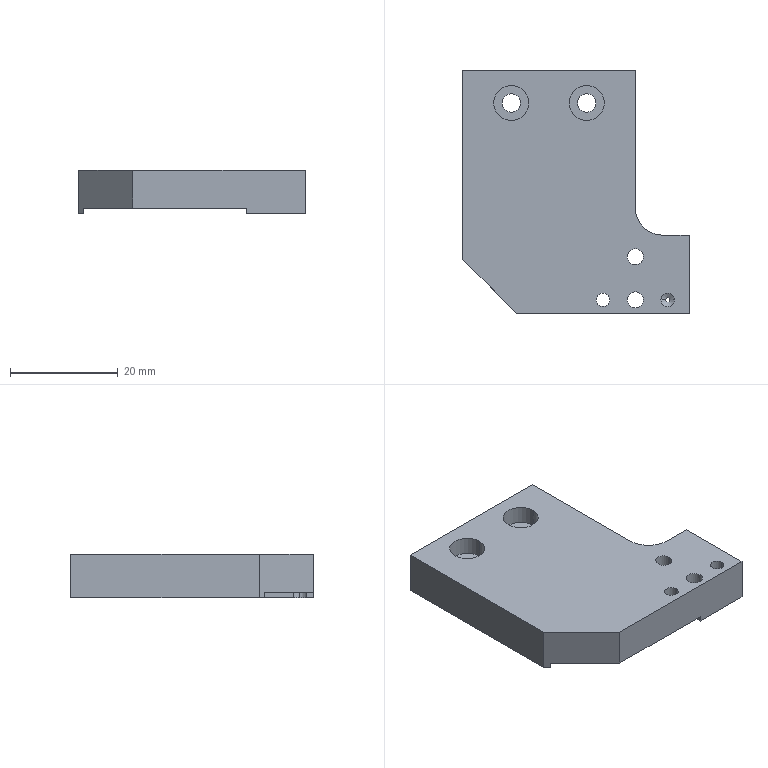Part | STEP file | 11-FG-E01811 | 1 solid | 36 faces | box 42 x 45 x 8 mm | volume 10535 mm3 | cylinder 17 | plane 17 | cone 2 | commonest cylinder face diameters 2.5 x4 3 x4 3.4 x4 6.5 x4 10 x1
STEP:
#1=CARTESIAN_POINT('',(8.75,-20.,1.));
#2=VERTEX_POINT('',#1);
#3=CARTESIAN_POINT('',(11.25,-20.,1.));
#4=VERTEX_POINT('',#3);
#5=CARTESIAN_POINT('',(10.,-20.,1.));
#6=DIRECTION('',(0.,0.,1.));
#7=DIRECTION('',(1.,0.,0.));
#8=AXIS2_PLACEMENT_3D('',#5,#6,#7);
#9=CIRCLE('',#8,1.25);
#10=EDGE_CURVE('',#2,#4,#9,.T.);
#11=ORIENTED_EDGE('',*,*,#10,.F.);
#12=CARTESIAN_POINT('',(8.75,-20.,8.));
#13=VERTEX_POINT('',#12);
#14=CARTESIAN_POINT('',(8.75,-20.,8.));
#15=DIRECTION('',(0.,0.,1.));
#16=VECTOR('',#15,1000.);
#17=LINE('',#14,#16);
#18=EDGE_CURVE('',#2,#13,#17,.T.);
#19=ORIENTED_EDGE('',*,*,#18,.T.);
#20=CARTESIAN_POINT('',(11.25,-20.,8.));
#21=VERTEX_POINT('',#20);
#22=CARTESIAN_POINT('',(10.,-20.,8.));
#23=DIRECTION('',(0.,0.,1.));
#24=DIRECTION('',(1.,0.,0.));
#25=AXIS2_PLACEMENT_3D('',#22,#23,#24);
#26=CIRCLE('',#25,1.25);
#27=EDGE_CURVE('',#13,#21,#26,.T.);
#28=ORIENTED_EDGE('',*,*,#27,.T.);
#29=CARTESIAN_POINT('',(11.25,-20.,8.));
#30=DIRECTION('',(0.,0.,1.));
#31=VECTOR('',#30,1000.);
#32=LINE('',#29,#31);
#33=EDGE_CURVE('',#4,#21,#32,.T.);
#34=ORIENTED_EDGE('',*,*,#33,.F.);
#35=EDGE_LOOP('',(#11,#19,#28,#34));
#36=FACE_OUTER_BOUND('',#35,.T.);
#37=CARTESIAN_POINT('',(10.,-20.,8.));
#38=DIRECTION('',(0.,0.,1.));
#39=DIRECTION('',(1.,0.,0.));
#40=AXIS2_PLACEMENT_3D('',#37,#38,#39);
#41=CYLINDRICAL_SURFACE('',#40,1.25);
#42=ADVANCED_FACE('',(#36),#41,.F.);
#43=CARTESIAN_POINT('',(20.75,-20.,0.5));
#44=VERTEX_POINT('',#43);
#45=CARTESIAN_POINT('',(23.25,-20.,0.5));
#46=VERTEX_POINT('',#45);
#47=CARTESIAN_POINT('',(22.,-20.,0.5));
#48=DIRECTION('',(0.,0.,1.));
#49=DIRECTION('',(1.,0.,0.));
#50=AXIS2_PLACEMENT_3D('',#47,#48,#49);
#51=CIRCLE('',#50,1.25);
#52=EDGE_CURVE('',#44,#46,#51,.T.);
#53=ORIENTED_EDGE('',*,*,#52,.F.);
#54=CARTESIAN_POINT('',(20.75,-20.,8.));
#55=VERTEX_POINT('',#54);
#56=CARTESIAN_POINT('',(20.75,-20.,8.));
#57=DIRECTION('',(0.,0.,1.));
#58=VECTOR('',#57,1000.);
#59=LINE('',#56,#58);
#60=EDGE_CURVE('',#44,#55,#59,.T.);
#61=ORIENTED_EDGE('',*,*,#60,.T.);
#62=CARTESIAN_POINT('',(23.25,-20.,8.));
#63=VERTEX_POINT('',#62);
#64=CARTESIAN_POINT('',(22.,-20.,8.));
#65=DIRECTION('',(0.,0.,1.));
#66=DIRECTION('',(1.,0.,0.));
#67=AXIS2_PLACEMENT_3D('',#64,#65,#66);
#68=CIRCLE('',#67,1.25);
#69=EDGE_CURVE('',#55,#63,#68,.T.);
#70=ORIENTED_EDGE('',*,*,#69,.T.);
#71=CARTESIAN_POINT('',(23.25,-20.,8.));
#72=DIRECTION('',(0.,0.,1.));
#73=VECTOR('',#72,1000.);
#74=LINE('',#71,#73);
#75=EDGE_CURVE('',#46,#63,#74,.T.);
#76=ORIENTED_EDGE('',*,*,#75,.F.);
#77=EDGE_LOOP('',(#53,#61,#70,#76));
#78=FACE_OUTER_BOUND('',#77,.T.);
#79=CARTESIAN_POINT('',(22.,-20.,8.));
#80=DIRECTION('',(0.,0.,1.));
#81=DIRECTION('',(1.,0.,0.));
#82=AXIS2_PLACEMENT_3D('',#79,#80,#81);
#83=CYLINDRICAL_SURFACE('',#82,1.25);
#84=ADVANCED_FACE('',(#78),#83,.F.);
#85=CARTESIAN_POINT('',(22.418,-20.,0.));
#86=VERTEX_POINT('',#85);
#87=CARTESIAN_POINT('',(21.582,-20.,0.));
#88=VERTEX_POINT('',#87);
#89=CARTESIAN_POINT('',(22.,-20.,0.));
#90=DIRECTION('',(0.,0.,-1.));
#91=DIRECTION('',(-1.,0.,0.));
#92=AXIS2_PLACEMENT_3D('',#89,#90,#91);
#93=CIRCLE('',#92,0.4179);
#94=EDGE_CURVE('',#86,#88,#93,.T.);
#95=ORIENTED_EDGE('',*,*,#94,.T.);
#96=CARTESIAN_POINT('',(20.75,-20.,0.5));
#97=DIRECTION('',(-0.8572,0.,0.515));
#98=VECTOR('',#97,1000.);
#99=LINE('',#96,#98);
#100=EDGE_CURVE('',#88,#44,#99,.T.);
#101=ORIENTED_EDGE('',*,*,#100,.T.);
#102=ORIENTED_EDGE('',*,*,#52,.T.);
#103=CARTESIAN_POINT('',(23.25,-20.,0.5));
#104=DIRECTION('',(0.8572,0.,0.515));
#105=VECTOR('',#104,1000.);
#106=LINE('',#103,#105);
#107=EDGE_CURVE('',#86,#46,#106,.T.);
#108=ORIENTED_EDGE('',*,*,#107,.F.);
#109=EDGE_LOOP('',(#95,#101,#102,#108));
#110=FACE_OUTER_BOUND('',#109,.T.);
#111=CARTESIAN_POINT('',(22.,-20.,0.5));
#112=DIRECTION('',(0.,0.,1.));
#113=DIRECTION('',(1.,0.,0.));
#114=AXIS2_PLACEMENT_3D('',#111,#112,#113);
#115=CONICAL_SURFACE('',#114,1.25,1.03);
#116=ADVANCED_FACE('',(#110),#115,.F.);
#117=CARTESIAN_POINT('',(14.5,-12.,1.));
#118=VERTEX_POINT('',#117);
#119=CARTESIAN_POINT('',(15.05,-13.161,1.));
#120=VERTEX_POINT('',#119);
#121=CARTESIAN_POINT('',(16.,-12.,1.));
#122=DIRECTION('',(0.,0.,1.));
#123=DIRECTION('',(1.,0.,0.));
#124=AXIS2_PLACEMENT_3D('',#121,#122,#123);
#125=CIRCLE('',#124,1.5);
#126=EDGE_CURVE('',#118,#120,#125,.T.);
#127=ORIENTED_EDGE('',*,*,#126,.F.);
#128=CARTESIAN_POINT('',(14.5,-12.,8.));
#129=VERTEX_POINT('',#128);
#130=CARTESIAN_POINT('',(14.5,-12.,8.));
#131=DIRECTION('',(0.,0.,1.));
#132=VECTOR('',#131,1000.);
#133=LINE('',#130,#132);
#134=EDGE_CURVE('',#118,#129,#133,.T.);
#135=ORIENTED_EDGE('',*,*,#134,.T.);
#136=CARTESIAN_POINT('',(17.5,-12.,8.));
#137=VERTEX_POINT('',#136);
#138=CARTESIAN_POINT('',(16.,-12.,8.));
#139=DIRECTION('',(0.,0.,1.));
#140=DIRECTION('',(1.,0.,0.));
#141=AXIS2_PLACEMENT_3D('',#138,#139,#140);
#142=CIRCLE('',#141,1.5);
#143=EDGE_CURVE('',#129,#137,#142,.T.);
#144=ORIENTED_EDGE('',*,*,#143,.T.);
#145=CARTESIAN_POINT('',(17.5,-12.,0.));
#146=VERTEX_POINT('',#145);
#147=CARTESIAN_POINT('',(17.5,-12.,8.));
#148=DIRECTION('',(0.,0.,1.));
#149=VECTOR('',#148,1000.);
#150=LINE('',#147,#149);
#151=EDGE_CURVE('',#146,#137,#150,.T.);
#152=ORIENTED_EDGE('',*,*,#151,.F.);
#153=CARTESIAN_POINT('',(15.05,-13.161,0.));
#154=VERTEX_POINT('',#153);
#155=CARTESIAN_POINT('',(16.,-12.,0.));
#156=DIRECTION('',(0.,0.,-1.));
#157=DIRECTION('',(-1.,0.,0.));
#158=AXIS2_PLACEMENT_3D('',#155,#156,#157);
#159=CIRCLE('',#158,1.5);
#160=EDGE_CURVE('',#146,#154,#159,.T.);
#161=ORIENTED_EDGE('',*,*,#160,.T.);
#162=CARTESIAN_POINT('',(15.05,-13.161,8.));
#163=DIRECTION('',(0.,0.,-1.));
#164=VECTOR('',#163,1000.);
#165=LINE('',#162,#164);
#166=EDGE_CURVE('',#120,#154,#165,.T.);
#167=ORIENTED_EDGE('',*,*,#166,.F.);
#168=EDGE_LOOP('',(#127,#135,#144,#152,#161,#167));
#169=FACE_OUTER_BOUND('',#168,.T.);
#170=CARTESIAN_POINT('',(16.,-12.,8.));
#171=DIRECTION('',(0.,0.,1.));
#172=DIRECTION('',(1.,0.,0.));
#173=AXIS2_PLACEMENT_3D('',#170,#171,#172);
#174=CYLINDRICAL_SURFACE('',#173,1.5);
#175=ADVANCED_FACE('',(#169),#174,.F.);
#176=CARTESIAN_POINT('',(14.5,-20.,1.));
#177=VERTEX_POINT('',#176);
#178=CARTESIAN_POINT('',(15.05,-21.161,1.));
#179=VERTEX_POINT('',#178);
#180=CARTESIAN_POINT('',(16.,-20.,1.));
#181=DIRECTION('',(0.,0.,1.));
#182=DIRECTION('',(1.,0.,0.));
#183=AXIS2_PLACEMENT_3D('',#180,#181,#182);
#184=CIRCLE('',#183,1.5);
#185=EDGE_CURVE('',#177,#179,#184,.T.);
#186=ORIENTED_EDGE('',*,*,#185,.F.);
#187=CARTESIAN_POINT('',(14.5,-20.,8.));
#188=VERTEX_POINT('',#187);
#189=CARTESIAN_POINT('',(14.5,-20.,8.));
#190=DIRECTION('',(0.,0.,1.));
#191=VECTOR('',#190,1000.);
#192=LINE('',#189,#191);
#193=EDGE_CURVE('',#177,#188,#192,.T.);
#194=ORIENTED_EDGE('',*,*,#193,.T.);
#195=CARTESIAN_POINT('',(17.5,-20.,8.));
#196=VERTEX_POINT('',#195);
#197=CARTESIAN_POINT('',(16.,-20.,8.));
#198=DIRECTION('',(0.,0.,1.));
#199=DIRECTION('',(1.,0.,0.));
#200=AXIS2_PLACEMENT_3D('',#197,#198,#199);
#201=CIRCLE('',#200,1.5);
#202=EDGE_CURVE('',#188,#196,#201,.T.);
#203=ORIENTED_EDGE('',*,*,#202,.T.);
#204=CARTESIAN_POINT('',(17.5,-20.,0.));
#205=VERTEX_POINT('',#204);
#206=CARTESIAN_POINT('',(17.5,-20.,8.));
#207=DIRECTION('',(0.,0.,1.));
#208=VECTOR('',#207,1000.);
#209=LINE('',#206,#208);
#210=EDGE_CURVE('',#205,#196,#209,.T.);
#211=ORIENTED_EDGE('',*,*,#210,.F.);
#212=CARTESIAN_POINT('',(15.05,-21.161,0.));
#213=VERTEX_POINT('',#212);
#214=CARTESIAN_POINT('',(16.,-20.,0.));
#215=DIRECTION('',(0.,0.,-1.));
#216=DIRECTION('',(-1.,0.,0.));
#217=AXIS2_PLACEMENT_3D('',#214,#215,#216);
#218=CIRCLE('',#217,1.5);
#219=EDGE_CURVE('',#205,#213,#218,.T.);
#220=ORIENTED_EDGE('',*,*,#219,.T.);
#221=CARTESIAN_POINT('',(15.05,-21.161,8.));
#222=DIRECTION('',(0.,0.,-1.));
#223=VECTOR('',#222,1000.);
#224=LINE('',#221,#223);
#225=EDGE_CURVE('',#179,#213,#224,.T.);
#226=ORIENTED_EDGE('',*,*,#225,.F.);
#227=EDGE_LOOP('',(#186,#194,#203,#211,#220,#226));
#228=FACE_OUTER_BOUND('',#227,.T.);
#229=CARTESIAN_POINT('',(16.,-20.,8.));
#230=DIRECTION('',(0.,0.,1.));
#231=DIRECTION('',(1.,0.,0.));
#232=AXIS2_PLACEMENT_3D('',#229,#230,#231);
#233=CYLINDRICAL_SURFACE('',#232,1.5);
#234=ADVANCED_FACE('',(#228),#233,.F.);
#235=CARTESIAN_POINT('',(3.75,16.5,4.6));
#236=VERTEX_POINT('',#235);
#237=CARTESIAN_POINT('',(10.25,16.5,4.6));
#238=VERTEX_POINT('',#237);
#239=CARTESIAN_POINT('',(7.,16.5,4.6));
#240=DIRECTION('',(0.,0.,1.));
#241=DIRECTION('',(1.,0.,0.));
#242=AXIS2_PLACEMENT_3D('',#239,#240,#241);
#243=CIRCLE('',#242,3.25);
#244=EDGE_CURVE('',#236,#238,#243,.T.);
#245=ORIENTED_EDGE('',*,*,#244,.F.);
#246=CARTESIAN_POINT('',(3.75,16.5,8.));
#247=VERTEX_POINT('',#246);
#248=CARTESIAN_POINT('',(3.75,16.5,8.));
#249=DIRECTION('',(0.,0.,1.));
#250=VECTOR('',#249,1000.);
#251=LINE('',#248,#250);
#252=EDGE_CURVE('',#236,#247,#251,.T.);
#253=ORIENTED_EDGE('',*,*,#252,.T.);
#254=CARTESIAN_POINT('',(10.25,16.5,8.));
#255=VERTEX_POINT('',#254);
#256=CARTESIAN_POINT('',(7.,16.5,8.));
#257=DIRECTION('',(0.,0.,1.));
#258=DIRECTION('',(1.,0.,0.));
#259=AXIS2_PLACEMENT_3D('',#256,#257,#258);
#260=CIRCLE('',#259,3.25);
#261=EDGE_CURVE('',#247,#255,#260,.T.);
#262=ORIENTED_EDGE('',*,*,#261,.T.);
#263=CARTESIAN_POINT('',(10.25,16.5,8.));
#264=DIRECTION('',(0.,0.,1.));
#265=VECTOR('',#264,1000.);
#266=LINE('',#263,#265);
#267=EDGE_CURVE('',#238,#255,#266,.T.);
#268=ORIENTED_EDGE('',*,*,#267,.F.);
#269=EDGE_LOOP('',(#245,#253,#262,#268));
#270=FACE_OUTER_BOUND('',#269,.T.);
#271=CARTESIAN_POINT('',(7.,16.5,8.));
#272=DIRECTION('',(0.,0.,1.));
#273=DIRECTION('',(1.,0.,0.));
#274=AXIS2_PLACEMENT_3D('',#271,#272,#273);
#275=CYLINDRICAL_SURFACE('',#274,3.25);
#276=ADVANCED_FACE('',(#270),#275,.F.);
#277=CARTESIAN_POINT('',(5.3,16.5,1.));
#278=VERTEX_POINT('',#277);
#279=CARTESIAN_POINT('',(8.7,16.5,1.));
#280=VERTEX_POINT('',#279);
#281=CARTESIAN_POINT('',(7.,16.5,1.));
#282=DIRECTION('',(0.,0.,1.));
#283=DIRECTION('',(1.,0.,0.));
#284=AXIS2_PLACEMENT_3D('',#281,#282,#283);
#285=CIRCLE('',#284,1.7);
#286=EDGE_CURVE('',#278,#280,#285,.T.);
#287=ORIENTED_EDGE('',*,*,#286,.F.);
#288=CARTESIAN_POINT('',(5.3,16.5,4.6));
#289=VERTEX_POINT('',#288);
#290=CARTESIAN_POINT('',(5.3,16.5,8.));
#291=DIRECTION('',(0.,0.,1.));
#292=VECTOR('',#291,1000.);
#293=LINE('',#290,#292);
#294=EDGE_CURVE('',#278,#289,#293,.T.);
#295=ORIENTED_EDGE('',*,*,#294,.T.);
#296=CARTESIAN_POINT('',(8.7,16.5,4.6));
#297=VERTEX_POINT('',#296);
#298=CARTESIAN_POINT('',(7.,16.5,4.6));
#299=DIRECTION('',(0.,0.,1.));
#300=DIRECTION('',(1.,0.,0.));
#301=AXIS2_PLACEMENT_3D('',#298,#299,#300);
#302=CIRCLE('',#301,1.7);
#303=EDGE_CURVE('',#289,#297,#302,.T.);
#304=ORIENTED_EDGE('',*,*,#303,.T.);
#305=CARTESIAN_POINT('',(8.7,16.5,8.));
#306=DIRECTION('',(0.,0.,1.));
#307=VECTOR('',#306,1000.);
#308=LINE('',#305,#307);
#309=EDGE_CURVE('',#280,#297,#308,.T.);
#310=ORIENTED_EDGE('',*,*,#309,.F.);
#311=EDGE_LOOP('',(#287,#295,#304,#310));
#312=FACE_OUTER_BOUND('',#311,.T.);
#313=CARTESIAN_POINT('',(7.,16.5,8.));
#314=DIRECTION('',(0.,0.,1.));
#315=DIRECTION('',(1.,0.,0.));
#316=AXIS2_PLACEMENT_3D('',#313,#314,#315);
#317=CYLINDRICAL_SURFACE('',#316,1.7);
#318=ADVANCED_FACE('',(#312),#317,.F.);
#319=CARTESIAN_POINT('',(-10.25,16.5,4.6));
#320=VERTEX_POINT('',#319);
#321=CARTESIAN_POINT('',(-3.75,16.5,4.6));
#322=VERTEX_POINT('',#321);
#323=CARTESIAN_POINT('',(-7.,16.5,4.6));
#324=DIRECTION('',(0.,0.,1.));
#325=DIRECTION('',(1.,0.,0.));
#326=AXIS2_PLACEMENT_3D('',#323,#324,#325);
#327=CIRCLE('',#326,3.25);
#328=EDGE_CURVE('',#320,#322,#327,.T.);
#329=ORIENTED_EDGE('',*,*,#328,.F.);
#330=CARTESIAN_POINT('',(-10.25,16.5,8.));
#331=VERTEX_POINT('',#330);
#332=CARTESIAN_POINT('',(-10.25,16.5,8.));
#333=DIRECTION('',(0.,0.,1.));
#334=VECTOR('',#333,1000.);
#335=LINE('',#332,#334);
#336=EDGE_CURVE('',#320,#331,#335,.T.);
#337=ORIENTED_EDGE('',*,*,#336,.T.);
#338=CARTESIAN_POINT('',(-3.75,16.5,8.));
#339=VERTEX_POINT('',#338);
#340=CARTESIAN_POINT('',(-7.,16.5,8.));
#341=DIRECTION('',(0.,0.,1.));
#342=DIRECTION('',(1.,0.,0.));
#343=AXIS2_PLACEMENT_3D('',#340,#341,#342);
#344=CIRCLE('',#343,3.25);
#345=EDGE_CURVE('',#331,#339,#344,.T.);
#346=ORIENTED_EDGE('',*,*,#345,.T.);
#347=CARTESIAN_POINT('',(-3.75,16.5,8.));
#348=DIRECTION('',(0.,0.,1.));
#349=VECTOR('',#348,1000.);
#350=LINE('',#347,#349);
#351=EDGE_CURVE('',#322,#339,#350,.T.);
#352=ORIENTED_EDGE('',*,*,#351,.F.);
#353=EDGE_LOOP('',(#329,#337,#346,#352));
#354=FACE_OUTER_BOUND('',#353,.T.);
#355=CARTESIAN_POINT('',(-7.,16.5,8.));
#356=DIRECTION('',(0.,0.,1.));
#357=DIRECTION('',(1.,0.,0.));
#358=AXIS2_PLACEMENT_3D('',#355,#356,#357);
#359=CYLINDRICAL_SURFACE('',#358,3.25);
#360=ADVANCED_FACE('',(#354),#359,.F.);
#361=CARTESIAN_POINT('',(-8.7,16.5,1.));
#362=VERTEX_POINT('',#361);
#363=CARTESIAN_POINT('',(-5.3,16.5,1.));
#364=VERTEX_POINT('',#363);
#365=CARTESIAN_POINT('',(-7.,16.5,1.));
#366=DIRECTION('',(0.,0.,1.));
#367=DIRECTION('',(1.,0.,0.));
#368=AXIS2_PLACEMENT_3D('',#365,#366,#367);
#369=CIRCLE('',#368,1.7);
#370=EDGE_CURVE('',#362,#364,#369,.T.);
#371=ORIENTED_EDGE('',*,*,#370,.F.);
#372=CARTESIAN_POINT('',(-8.7,16.5,4.6));
#373=VERTEX_POINT('',#372);
#374=CARTESIAN_POINT('',(-8.7,16.5,8.));
#375=DIRECTION('',(0.,0.,1.));
#376=VECTOR('',#375,1000.);
#377=LINE('',#374,#376);
#378=EDGE_CURVE('',#362,#373,#377,.T.);
#379=ORIENTED_EDGE('',*,*,#378,.T.);
#380=CARTESIAN_POINT('',(-5.3,16.5,4.6));
#381=VERTEX_POINT('',#380);
#382=CARTESIAN_POINT('',(-7.,16.5,4.6));
#383=DIRECTION('',(0.,0.,1.));
#384=DIRECTION('',(1.,0.,0.));
#385=AXIS2_PLACEMENT_3D('',#382,#383,#384);
#386=CIRCLE('',#385,1.7);
#387=EDGE_CURVE('',#373,#381,#386,.T.);
#388=ORIENTED_EDGE('',*,*,#387,.T.);
#389=CARTESIAN_POINT('',(-5.3,16.5,8.));
#390=DIRECTION('',(0.,0.,1.));
#391=VECTOR('',#390,1000.);
#392=LINE('',#389,#391);
#393=EDGE_CURVE('',#364,#381,#392,.T.);
#394=ORIENTED_EDGE('',*,*,#393,.F.);
#395=EDGE_LOOP('',(#371,#379,#388,#394));
#396=FACE_OUTER_BOUND('',#395,.T.);
#397=CARTESIAN_POINT('',(-7.,16.5,8.));
#398=DIRECTION('',(0.,0.,1.));
#399=DIRECTION('',(1.,0.,0.));
#400=AXIS2_PLACEMENT_3D('',#397,#398,#399);
#401=CYLINDRICAL_SURFACE('',#400,1.7);
#402=ADVANCED_FACE('',(#396),#401,.F.);
#403=CARTESIAN_POINT('',(15.05,22.5,0.));
#404=VERTEX_POINT('',#403);
#405=CARTESIAN_POINT('',(15.05,-10.839,0.));
#406=VERTEX_POINT('',#405);
#407=CARTESIAN_POINT('',(15.05,0.,0.));
#408=DIRECTION('',(0.,-1.,0.));
#409=VECTOR('',#408,1000.);
#410=LINE('',#407,#409);
#411=EDGE_CURVE('',#404,#406,#410,.T.);
#412=ORIENTED_EDGE('',*,*,#411,.T.);
#413=CARTESIAN_POINT('',(15.05,-10.839,1.));
#414=VERTEX_POINT('',#413);
#415=CARTESIAN_POINT('',(15.05,-10.839,8.));
#416=DIRECTION('',(0.,0.,1.));
#417=VECTOR('',#416,1000.);
#418=LINE('',#415,#417);
#419=EDGE_CURVE('',#406,#414,#418,.T.);
#420=ORIENTED_EDGE('',*,*,#419,.T.);
#421=CARTESIAN_POINT('',(15.05,22.5,1.));
#422=VERTEX_POINT('',#421);
#423=CARTESIAN_POINT('',(15.05,-33.5,1.));
#424=DIRECTION('',(0.,1.,0.));
#425=VECTOR('',#424,1000.);
#426=LINE('',#423,#425);
#427=EDGE_CURVE('',#414,#422,#426,.T.);
#428=ORIENTED_EDGE('',*,*,#427,.T.);
#429=CARTESIAN_POINT('',(15.05,22.5,1.));
#430=DIRECTION('',(0.,0.,-1.));
#431=VECTOR('',#430,1000.);
#432=LINE('',#429,#431);
#433=EDGE_CURVE('',#422,#404,#432,.T.);
#434=ORIENTED_EDGE('',*,*,#433,.T.);
#435=EDGE_LOOP('',(#412,#420,#428,#434));
#436=FACE_OUTER_BOUND('',#435,.T.);
#437=CARTESIAN_POINT('',(15.05,-33.5,1.));
#438=DIRECTION('',(1.,0.,0.));
#439=DIRECTION('',(0.,0.,-1.));
#440=AXIS2_PLACEMENT_3D('',#437,#438,#439);
#441=PLANE('',#440);
#442=ADVANCED_FACE('',(#436),#441,.F.);
#443=CARTESIAN_POINT('',(15.05,-18.839,1.));
#444=VERTEX_POINT('',#443);
#445=CARTESIAN_POINT('',(15.05,-33.5,1.));
#446=DIRECTION('',(0.,1.,0.));
#447=VECTOR('',#446,1000.);
#448=LINE('',#445,#447);
#449=EDGE_CURVE('',#444,#120,#448,.T.);
#450=ORIENTED_EDGE('',*,*,#449,.T.);
#451=ORIENTED_EDGE('',*,*,#166,.T.);
#452=CARTESIAN_POINT('',(15.05,-18.839,0.));
#453=VERTEX_POINT('',#452);
#454=CARTESIAN_POINT('',(15.05,0.,0.));
#455=DIRECTION('',(0.,-1.,0.));
#456=VECTOR('',#455,1000.);
#457=LINE('',#454,#456);
#458=EDGE_CURVE('',#154,#453,#457,.T.);
#459=ORIENTED_EDGE('',*,*,#458,.T.);
#460=CARTESIAN_POINT('',(15.05,-18.839,8.));
#461=DIRECTION('',(0.,0.,1.));
#462=VECTOR('',#461,1000.);
#463=LINE('',#460,#462);
#464=EDGE_CURVE('',#453,#444,#463,.T.);
#465=ORIENTED_EDGE('',*,*,#464,.T.);
#466=EDGE_LOOP('',(#450,#451,#459,#465));
#467=FACE_OUTER_BOUND('',#466,.T.);
#468=CARTESIAN_POINT('',(15.05,-33.5,1.));
#469=DIRECTION('',(1.,0.,0.));
#470=DIRECTION('',(0.,0.,-1.));
#471=AXIS2_PLACEMENT_3D('',#468,#469,#470);
#472=PLANE('',#471);
#473=ADVANCED_FACE('',(#467),#472,.F.);
#474=CARTESIAN_POINT('',(16.,-3.,8.));
#475=VERTEX_POINT('',#474);
#476=CARTESIAN_POINT('',(16.,22.5,8.));
#477=VERTEX_POINT('',#476);
#478=CARTESIAN_POINT('',(16.,-22.5,8.));
#479=DIRECTION('',(0.,1.,0.));
#480=VECTOR('',#479,1000.);
#481=LINE('',#478,#480);
#482=EDGE_CURVE('',#475,#477,#481,.T.);
#483=ORIENTED_EDGE('',*,*,#482,.F.);
#484=CARTESIAN_POINT('',(16.,-3.,0.));
#485=VERTEX_POINT('',#484);
#486=CARTESIAN_POINT('',(16.,-3.,8.));
#487=DIRECTION('',(0.,0.,-1.));
#488=VECTOR('',#487,1000.);
#489=LINE('',#486,#488);
#490=EDGE_CURVE('',#475,#485,#489,.T.);
#491=ORIENTED_EDGE('',*,*,#490,.T.);
#492=CARTESIAN_POINT('',(16.,22.5,0.));
#493=VERTEX_POINT('',#492);
#494=CARTESIAN_POINT('',(16.,-22.5,0.));
#495=DIRECTION('',(0.,1.,0.));
#496=VECTOR('',#495,1000.);
#497=LINE('',#494,#496);
#498=EDGE_CURVE('',#485,#493,#497,.T.);
#499=ORIENTED_EDGE('',*,*,#498,.T.);
#500=CARTESIAN_POINT('',(16.,22.5,8.));
#501=DIRECTION('',(0.,0.,-1.));
#502=VECTOR('',#501,1000.);
#503=LINE('',#500,#502);
#504=EDGE_CURVE('',#477,#493,#503,.T.);
#505=ORIENTED_EDGE('',*,*,#504,.F.);
#506=EDGE_LOOP('',(#483,#491,#499,#505));
#507=FACE_OUTER_BOUND('',#506,.T.);
#508=CARTESIAN_POINT('',(16.,-22.5,8.));
#509=DIRECTION('',(-1.,0.,0.));
#510=DIRECTION('',(0.,0.,1.));
#511=AXIS2_PLACEMENT_3D('',#508,#509,#510);
#512=PLANE('',#511);
#513=ADVANCED_FACE('',(#507),#512,.F.);
#514=ORIENTED_EDGE('',*,*,#94,.F.);
#515=CARTESIAN_POINT('',(22.,-20.,0.));
#516=DIRECTION('',(0.,0.,-1.));
#517=DIRECTION('',(-1.,0.,0.));
#518=AXIS2_PLACEMENT_3D('',#515,#516,#517);
#519=CIRCLE('',#518,0.4179);
#520=EDGE_CURVE('',#88,#86,#519,.T.);
#521=ORIENTED_EDGE('',*,*,#520,.F.);
#522=EDGE_LOOP('',(#514,#521));
#523=FACE_BOUND('',#522,.T.);
#524=CARTESIAN_POINT('',(16.,-12.,0.));
#525=DIRECTION('',(0.,0.,-1.));
#526=DIRECTION('',(-1.,0.,0.));
#527=AXIS2_PLACEMENT_3D('',#524,#525,#526);
#528=CIRCLE('',#527,1.5);
#529=EDGE_CURVE('',#406,#146,#528,.T.);
#530=ORIENTED_EDGE('',*,*,#529,.F.);
#531=ORIENTED_EDGE('',*,*,#411,.F.);
#532=CARTESIAN_POINT('',(-16.,22.5,0.));
#533=DIRECTION('',(-1.,0.,0.));
#534=VECTOR('',#533,1000.);
#535=LINE('',#532,#534);
#536=EDGE_CURVE('',#493,#404,#535,.T.);
#537=ORIENTED_EDGE('',*,*,#536,.F.);
#538=ORIENTED_EDGE('',*,*,#498,.F.);
#539=CARTESIAN_POINT('',(21.,-8.,0.));
#540=VERTEX_POINT('',#539);
#541=CARTESIAN_POINT('',(21.,-3.,0.));
#542=DIRECTION('',(0.,0.,1.));
#543=DIRECTION('',(-1.,0.,0.));
#544=AXIS2_PLACEMENT_3D('',#541,#542,#543);
#545=CIRCLE('',#544,5.);
#546=EDGE_CURVE('',#485,#540,#545,.T.);
#547=ORIENTED_EDGE('',*,*,#546,.T.);
#548=CARTESIAN_POINT('',(26.,-8.,0.));
#549=VERTEX_POINT('',#548);
#550=CARTESIAN_POINT('',(16.,-8.,0.));
#551=DIRECTION('',(-1.,0.,0.));
#552=VECTOR('',#551,1000.);
#553=LINE('',#550,#552);
#554=EDGE_CURVE('',#549,#540,#553,.T.);
#555=ORIENTED_EDGE('',*,*,#554,.F.);
#556=CARTESIAN_POINT('',(26.,-22.5,0.));
#557=VERTEX_POINT('',#556);
#558=CARTESIAN_POINT('',(26.,-22.5,0.));
#559=DIRECTION('',(0.,1.,0.));
#560=VECTOR('',#559,1000.);
#561=LINE('',#558,#560);
#562=EDGE_CURVE('',#557,#549,#561,.T.);
#563=ORIENTED_EDGE('',*,*,#562,.F.);
#564=CARTESIAN_POINT('',(15.05,-22.5,0.));
#565=VERTEX_POINT('',#564);
#566=CARTESIAN_POINT('',(-16.,-22.5,0.));
#567=DIRECTION('',(1.,0.,0.));
#568=VECTOR('',#567,1000.);
#569=LINE('',#566,#568);
#570=EDGE_CURVE('',#565,#557,#569,.T.);
#571=ORIENTED_EDGE('',*,*,#570,.F.);
#572=CARTESIAN_POINT('',(15.05,0.,0.));
#573=DIRECTION('',(0.,-1.,0.));
#574=VECTOR('',#573,1000.);
#575=LINE('',#572,#574);
#576=EDGE_CURVE('',#213,#565,#575,.T.);
#577=ORIENTED_EDGE('',*,*,#576,.F.);
#578=ORIENTED_EDGE('',*,*,#219,.F.);
#579=CARTESIAN_POINT('',(16.,-20.,0.));
#580=DIRECTION('',(0.,0.,-1.));
#581=DIRECTION('',(-1.,0.,0.));
#582=AXIS2_PLACEMENT_3D('',#579,#580,#581);
#583=CIRCLE('',#582,1.5);
#584=EDGE_CURVE('',#453,#205,#583,.T.);
#585=ORIENTED_EDGE('',*,*,#584,.F.);
#586=ORIENTED_EDGE('',*,*,#458,.F.);
#587=ORIENTED_EDGE('',*,*,#160,.F.);
#588=EDGE_LOOP('',(#530,#531,#537,#538,#547,#555,#563,#571,#577,#578,#585,#586,#587));
#589=FACE_OUTER_BOUND('',#588,.T.);
#590=CARTESIAN_POINT('',(0.,0.,0.));
#591=DIRECTION('',(0.,0.,-1.));
#592=DIRECTION('',(-1.,0.,0.));
#593=AXIS2_PLACEMENT_3D('',#590,#591,#592);
#594=PLANE('',#593);
#595=ADVANCED_FACE('',(#523,#589),#594,.T.);
#596=ORIENTED_EDGE('',*,*,#536,.T.);
#597=ORIENTED_EDGE('',*,*,#433,.F.);
#598=CARTESIAN_POINT('',(-15.05,22.5,1.));
#599=VERTEX_POINT('',#598);
#600=CARTESIAN_POINT('',(15.05,22.5,1.));
#601=DIRECTION('',(1.,0.,0.));
#602=VECTOR('',#601,1000.);
#603=LINE('',#600,#602);
#604=EDGE_CURVE('',#599,#422,#603,.T.);
#605=ORIENTED_EDGE('',*,*,#604,.F.);
#606=CARTESIAN_POINT('',(-15.05,22.5,0.));
#607=VERTEX_POINT('',#606);
#608=CARTESIAN_POINT('',(-15.05,22.5,1.));
#609=DIRECTION('',(0.,0.,1.));
#610=VECTOR('',#609,1000.);
#611=LINE('',#608,#610);
#612=EDGE_CURVE('',#607,#599,#611,.T.);
#613=ORIENTED_EDGE('',*,*,#612,.F.);
#614=CARTESIAN_POINT('',(-16.,22.5,0.));
#615=VERTEX_POINT('',#614);
#616=CARTESIAN_POINT('',(-16.,22.5,0.));
#617=DIRECTION('',(-1.,0.,0.));
#618=VECTOR('',#617,1000.);
#619=LINE('',#616,#618);
#620=EDGE_CURVE('',#607,#615,#619,.T.);
#621=ORIENTED_EDGE('',*,*,#620,.T.);
#622=CARTESIAN_POINT('',(-16.,22.5,8.));
#623=VERTEX_POINT('',#622);
#624=CARTESIAN_POINT('',(-16.,22.5,8.));
#625=DIRECTION('',(0.,0.,-1.));
#626=VECTOR('',#625,1000.);
#627=LINE('',#624,#626);
#628=EDGE_CURVE('',#623,#615,#627,.T.);
#629=ORIENTED_EDGE('',*,*,#628,.F.);
#630=CARTESIAN_POINT('',(-16.,22.5,8.));
#631=DIRECTION('',(-1.,0.,0.));
#632=VECTOR('',#631,1000.);
#633=LINE('',#630,#632);
#634=EDGE_CURVE('',#477,#623,#633,.T.);
#635=ORIENTED_EDGE('',*,*,#634,.F.);
#636=ORIENTED_EDGE('',*,*,#504,.T.);
#637=EDGE_LOOP('',(#596,#597,#605,#613,#621,#629,#635,#636));
#638=FACE_OUTER_BOUND('',#637,.T.);
#639=CARTESIAN_POINT('',(-16.,22.5,8.));
#640=DIRECTION('',(0.,-1.,0.));
#641=DIRECTION('',(0.,0.,-1.));
#642=AXIS2_PLACEMENT_3D('',#639,#640,#641);
#643=PLANE('',#642);
#644=ADVANCED_FACE('',(#638),#643,.F.);
#645=CARTESIAN_POINT('',(-16.,-12.5,0.));
#646=VERTEX_POINT('',#645);
#647=CARTESIAN_POINT('',(-16.,-22.5,0.));
#648=DIRECTION('',(0.,-1.,0.));
#649=VECTOR('',#648,1000.);
#650=LINE('',#647,#649);
#651=EDGE_CURVE('',#615,#646,#650,.T.);
#652=ORIENTED_EDGE('',*,*,#651,.T.);
#653=CARTESIAN_POINT('',(-16.,-12.5,8.));
#654=VERTEX_POINT('',#653);
#655=CARTESIAN_POINT('',(-16.,-12.5,8.));
#656=DIRECTION('',(0.,0.,1.));
#657=VECTOR('',#656,1000.);
#658=LINE('',#655,#657);
#659=EDGE_CURVE('',#646,#654,#658,.T.);
#660=ORIENTED_EDGE('',*,*,#659,.T.);
#661=CARTESIAN_POINT('',(-16.,-22.5,8.));
#662=DIRECTION('',(0.,-1.,0.));
#663=VECTOR('',#662,1000.);
#664=LINE('',#661,#663);
#665=EDGE_CURVE('',#623,#654,#664,.T.);
#666=ORIENTED_EDGE('',*,*,#665,.F.);
#667=ORIENTED_EDGE('',*,*,#628,.T.);
#668=EDGE_LOOP('',(#652,#660,#666,#667));
#669=FACE_OUTER_BOUND('',#668,.T.);
#670=CARTESIAN_POINT('',(-16.,-22.5,8.));
#671=DIRECTION('',(1.,0.,0.));
#672=DIRECTION('',(0.,0.,-1.));
#673=AXIS2_PLACEMENT_3D('',#670,#671,#672);
#674=PLANE('',#673);
#675=ADVANCED_FACE('',(#669),#674,.F.);
#676=CARTESIAN_POINT('',(-6.,-22.5,8.));
#677=VERTEX_POINT('',#676);
#678=CARTESIAN_POINT('',(26.,-22.5,8.));
#679=VERTEX_POINT('',#678);
#680=CARTESIAN_POINT('',(-16.,-22.5,8.));
#681=DIRECTION('',(1.,0.,0.));
#682=VECTOR('',#681,1000.);
#683=LINE('',#680,#682);
#684=EDGE_CURVE('',#677,#679,#683,.T.);
#685=ORIENTED_EDGE('',*,*,#684,.F.);
#686=CARTESIAN_POINT('',(-6.,-22.5,1.));
#687=VERTEX_POINT('',#686);
#688=CARTESIAN_POINT('',(-6.,-22.5,8.));
#689=DIRECTION('',(0.,0.,-1.));
#690=VECTOR('',#689,1000.);
#691=LINE('',#688,#690);
#692=EDGE_CURVE('',#677,#687,#691,.T.);
#693=ORIENTED_EDGE('',*,*,#692,.T.);
#694=CARTESIAN_POINT('',(15.05,-22.5,1.));
#695=VERTEX_POINT('',#694);
#696=CARTESIAN_POINT('',(-16.,-22.5,1.));
#697=DIRECTION('',(1.,0.,0.));
#698=VECTOR('',#697,1000.);
#699=LINE('',#696,#698);
#700=EDGE_CURVE('',#687,#695,#699,.T.);
#701=ORIENTED_EDGE('',*,*,#700,.T.);
#702=CARTESIAN_POINT('',(15.05,-22.5,8.));
#703=DIRECTION('',(0.,0.,-1.));
#704=VECTOR('',#703,1000.);
#705=LINE('',#702,#704);
#706=EDGE_CURVE('',#695,#565,#705,.T.);
#707=ORIENTED_EDGE('',*,*,#706,.T.);
#708=ORIENTED_EDGE('',*,*,#570,.T.);
#709=CARTESIAN_POINT('',(26.,-22.5,-17.614));
#710=DIRECTION('',(0.,0.,1.));
#711=VECTOR('',#710,1000.);
#712=LINE('',#709,#711);
#713=EDGE_CURVE('',#557,#679,#712,.T.);
#714=ORIENTED_EDGE('',*,*,#713,.T.);
#715=EDGE_LOOP('',(#685,#693,#701,#707,#708,#714));
#716=FACE_OUTER_BOUND('',#715,.T.);
#717=CARTESIAN_POINT('',(-16.,-22.5,8.));
#718=DIRECTION('',(0.,1.,0.));
#719=DIRECTION('',(0.,0.,1.));
#720=AXIS2_PLACEMENT_3D('',#717,#718,#719);
#721=PLANE('',#720);
#722=ADVANCED_FACE('',(#716),#721,.F.);
#723=CARTESIAN_POINT('',(10.,-20.,8.));
#724=DIRECTION('',(0.,0.,1.));
#725=DIRECTION('',(1.,0.,0.));
#726=AXIS2_PLACEMENT_3D('',#723,#724,#725);
#727=CIRCLE('',#726,1.25);
#728=EDGE_CURVE('',#21,#13,#727,.T.);
#729=ORIENTED_EDGE('',*,*,#728,.F.);
#730=ORIENTED_EDGE('',*,*,#27,.F.);
#731=EDGE_LOOP('',(#729,#730));
#732=FACE_BOUND('',#731,.T.);
#733=CARTESIAN_POINT('',(22.,-20.,8.));
#734=DIRECTION('',(0.,0.,1.));
#735=DIRECTION('',(1.,0.,0.));
#736=AXIS2_PLACEMENT_3D('',#733,#734,#735);
#737=CIRCLE('',#736,1.25);
#738=EDGE_CURVE('',#63,#55,#737,.T.);
#739=ORIENTED_EDGE('',*,*,#738,.F.);
#740=ORIENTED_EDGE('',*,*,#69,.F.);
#741=EDGE_LOOP('',(#739,#740));
#742=FACE_BOUND('',#741,.T.);
#743=CARTESIAN_POINT('',(16.,-12.,8.));
#744=DIRECTION('',(0.,0.,1.));
#745=DIRECTION('',(1.,0.,0.));
#746=AXIS2_PLACEMENT_3D('',#743,#744,#745);
#747=CIRCLE('',#746,1.5);
#748=EDGE_CURVE('',#137,#129,#747,.T.);
#749=ORIENTED_EDGE('',*,*,#748,.F.);
#750=ORIENTED_EDGE('',*,*,#143,.F.);
#751=EDGE_LOOP('',(#749,#750));
#752=FACE_BOUND('',#751,.T.);
#753=CARTESIAN_POINT('',(16.,-20.,8.));
#754=DIRECTION('',(0.,0.,1.));
#755=DIRECTION('',(1.,0.,0.));
#756=AXIS2_PLACEMENT_3D('',#753,#754,#755);
#757=CIRCLE('',#756,1.5);
#758=EDGE_CURVE('',#196,#188,#757,.T.);
#759=ORIENTED_EDGE('',*,*,#758,.F.);
#760=ORIENTED_EDGE('',*,*,#202,.F.);
#761=EDGE_LOOP('',(#759,#760));
#762=FACE_BOUND('',#761,.T.);
#763=CARTESIAN_POINT('',(7.,16.5,8.));
#764=DIRECTION('',(0.,0.,1.));
#765=DIRECTION('',(1.,0.,0.));
#766=AXIS2_PLACEMENT_3D('',#763,#764,#765);
#767=CIRCLE('',#766,3.25);
#768=EDGE_CURVE('',#255,#247,#767,.T.);
#769=ORIENTED_EDGE('',*,*,#768,.F.);
#770=ORIENTED_EDGE('',*,*,#261,.F.);
#771=EDGE_LOOP('',(#769,#770));
#772=FACE_BOUND('',#771,.T.);
#773=CARTESIAN_POINT('',(-7.,16.5,8.));
#774=DIRECTION('',(0.,0.,1.));
#775=DIRECTION('',(1.,0.,0.));
#776=AXIS2_PLACEMENT_3D('',#773,#774,#775);
#777=CIRCLE('',#776,3.25);
#778=EDGE_CURVE('',#339,#331,#777,.T.);
#779=ORIENTED_EDGE('',*,*,#778,.F.);
#780=ORIENTED_EDGE('',*,*,#345,.F.);
#781=EDGE_LOOP('',(#779,#780));
#782=FACE_BOUND('',#781,.T.);
#783=ORIENTED_EDGE('',*,*,#665,.T.);
#784=CARTESIAN_POINT('',(-6.,-22.5,8.));
#785=DIRECTION('',(0.7071,-0.7071,0.));
#786=VECTOR('',#785,1000.);
#787=LINE('',#784,#786);
#788=EDGE_CURVE('',#654,#677,#787,.T.);
#789=ORIENTED_EDGE('',*,*,#788,.T.);
#790=ORIENTED_EDGE('',*,*,#684,.T.);
#791=CARTESIAN_POINT('',(26.,-8.,8.));
#792=VERTEX_POINT('',#791);
#793=CARTESIAN_POINT('',(26.,-22.5,8.));
#794=DIRECTION('',(0.,1.,0.));
#795=VECTOR('',#794,1000.);
#796=LINE('',#793,#795);
#797=EDGE_CURVE('',#679,#792,#796,.T.);
#798=ORIENTED_EDGE('',*,*,#797,.T.);
#799=CARTESIAN_POINT('',(21.,-8.,8.));
#800=VERTEX_POINT('',#799);
#801=CARTESIAN_POINT('',(16.,-8.,8.));
#802=DIRECTION('',(-1.,0.,0.));
#803=VECTOR('',#802,1000.);
#804=LINE('',#801,#803);
#805=EDGE_CURVE('',#792,#800,#804,.T.);
#806=ORIENTED_EDGE('',*,*,#805,.T.);
#807=CARTESIAN_POINT('',(21.,-3.,8.));
#808=DIRECTION('',(0.,0.,-1.));
#809=DIRECTION('',(-1.,0.,0.));
#810=AXIS2_PLACEMENT_3D('',#807,#808,#809);
#811=CIRCLE('',#810,5.);
#812=EDGE_CURVE('',#800,#475,#811,.T.);
#813=ORIENTED_EDGE('',*,*,#812,.T.);
#814=ORIENTED_EDGE('',*,*,#482,.T.);
#815=ORIENTED_EDGE('',*,*,#634,.T.);
#816=EDGE_LOOP('',(#783,#789,#790,#798,#806,#813,#814,#815));
#817=FACE_OUTER_BOUND('',#816,.T.);
#818=CARTESIAN_POINT('',(0.,0.,8.));
#819=DIRECTION('',(0.,0.,-1.));
#820=DIRECTION('',(-1.,0.,0.));
#821=AXIS2_PLACEMENT_3D('',#818,#819,#820);
#822=PLANE('',#821);
#823=ADVANCED_FACE('',(#732,#742,#752,#762,#772,#782,#817),#822,.F.);
#824=CARTESIAN_POINT('',(-15.05,-13.45,0.));
#825=VERTEX_POINT('',#824);
#826=CARTESIAN_POINT('',(-15.05,0.,0.));
#827=DIRECTION('',(0.,1.,0.));
#828=VECTOR('',#827,1000.);
#829=LINE('',#826,#828);
#830=EDGE_CURVE('',#825,#607,#829,.T.);
#831=ORIENTED_EDGE('',*,*,#830,.F.);
#832=CARTESIAN_POINT('',(-14.25,-14.25,0.));
#833=DIRECTION('',(-0.7071,0.7071,0.));
#834=VECTOR('',#833,1000.);
#835=LINE('',#832,#834);
#836=EDGE_CURVE('',#825,#646,#835,.T.);
#837=ORIENTED_EDGE('',*,*,#836,.T.);
#838=ORIENTED_EDGE('',*,*,#651,.F.);
#839=ORIENTED_EDGE('',*,*,#620,.F.);
#840=EDGE_LOOP('',(#831,#837,#838,#839));
#841=FACE_OUTER_BOUND('',#840,.T.);
#842=CARTESIAN_POINT('',(0.,0.,0.));
#843=DIRECTION('',(0.,0.,-1.));
#844=DIRECTION('',(-1.,0.,0.));
#845=AXIS2_PLACEMENT_3D('',#842,#843,#844);
#846=PLANE('',#845);
#847=ADVANCED_FACE('',(#841),#846,.T.);
#848=CARTESIAN_POINT('',(10.,-20.,1.));
#849=DIRECTION('',(0.,0.,1.));
#850=DIRECTION('',(1.,0.,0.));
#851=AXIS2_PLACEMENT_3D('',#848,#849,#850);
#852=CIRCLE('',#851,1.25);
#853=EDGE_CURVE('',#4,#2,#852,.T.);
#854=ORIENTED_EDGE('',*,*,#853,.T.);
#855=ORIENTED_EDGE('',*,*,#10,.T.);
#856=EDGE_LOOP('',(#854,#855));
#857=FACE_BOUND('',#856,.T.);
#858=CARTESIAN_POINT('',(7.,16.5,1.));
#859=DIRECTION('',(0.,0.,1.));
#860=DIRECTION('',(1.,0.,0.));
#861=AXIS2_PLACEMENT_3D('',#858,#859,#860);
#862=CIRCLE('',#861,1.7);
#863=EDGE_CURVE('',#280,#278,#862,.T.);
#864=ORIENTED_EDGE('',*,*,#863,.T.);
#865=ORIENTED_EDGE('',*,*,#286,.T.);
#866=EDGE_LOOP('',(#864,#865));
#867=FACE_BOUND('',#866,.T.);
#868=CARTESIAN_POINT('',(-7.,16.5,1.));
#869=DIRECTION('',(0.,0.,1.));
#870=DIRECTION('',(1.,0.,0.));
#871=AXIS2_PLACEMENT_3D('',#868,#869,#870);
#872=CIRCLE('',#871,1.7);
#873=EDGE_CURVE('',#364,#362,#872,.T.);
#874=ORIENTED_EDGE('',*,*,#873,.T.);
#875=ORIENTED_EDGE('',*,*,#370,.T.);
#876=EDGE_LOOP('',(#874,#875));
#877=FACE_BOUND('',#876,.T.);
#878=ORIENTED_EDGE('',*,*,#700,.F.);
#879=CARTESIAN_POINT('',(-15.05,-13.45,1.));
#880=VERTEX_POINT('',#879);
#881=CARTESIAN_POINT('',(-6.,-22.5,1.));
#882=DIRECTION('',(-0.7071,0.7071,0.));
#883=VECTOR('',#882,1000.);
#884=LINE('',#881,#883);
#885=EDGE_CURVE('',#687,#880,#884,.T.);
#886=ORIENTED_EDGE('',*,*,#885,.T.);
#887=CARTESIAN_POINT('',(-15.05,-33.5,1.));
#888=DIRECTION('',(0.,1.,0.));
#889=VECTOR('',#888,1000.);
#890=LINE('',#887,#889);
#891=EDGE_CURVE('',#880,#599,#890,.T.);
#892=ORIENTED_EDGE('',*,*,#891,.T.);
#893=ORIENTED_EDGE('',*,*,#604,.T.);
#894=ORIENTED_EDGE('',*,*,#427,.F.);
#895=CARTESIAN_POINT('',(16.,-12.,1.));
#896=DIRECTION('',(0.,0.,1.));
#897=DIRECTION('',(1.,0.,0.));
#898=AXIS2_PLACEMENT_3D('',#895,#896,#897);
#899=CIRCLE('',#898,1.5);
#900=EDGE_CURVE('',#414,#118,#899,.T.);
#901=ORIENTED_EDGE('',*,*,#900,.T.);
#902=ORIENTED_EDGE('',*,*,#126,.T.);
#903=ORIENTED_EDGE('',*,*,#449,.F.);
#904=CARTESIAN_POINT('',(16.,-20.,1.));
#905=DIRECTION('',(0.,0.,1.));
#906=DIRECTION('',(1.,0.,0.));
#907=AXIS2_PLACEMENT_3D('',#904,#905,#906);
#908=CIRCLE('',#907,1.5);
#909=EDGE_CURVE('',#444,#177,#908,.T.);
#910=ORIENTED_EDGE('',*,*,#909,.T.);
#911=ORIENTED_EDGE('',*,*,#185,.T.);
#912=CARTESIAN_POINT('',(15.05,-33.5,1.));
#913=DIRECTION('',(0.,1.,0.));
#914=VECTOR('',#913,1000.);
#915=LINE('',#912,#914);
#916=EDGE_CURVE('',#695,#179,#915,.T.);
#917=ORIENTED_EDGE('',*,*,#916,.F.);
#918=EDGE_LOOP('',(#878,#886,#892,#893,#894,#901,#902,#903,#910,#911,#917));
#919=FACE_OUTER_BOUND('',#918,.T.);
#920=CARTESIAN_POINT('',(15.05,-33.5,1.));
#921=DIRECTION('',(0.,0.,1.));
#922=DIRECTION('',(1.,0.,0.));
#923=AXIS2_PLACEMENT_3D('',#920,#921,#922);
#924=PLANE('',#923);
#925=ADVANCED_FACE('',(#857,#867,#877,#919),#924,.F.);
#926=ORIENTED_EDGE('',*,*,#916,.T.);
#927=ORIENTED_EDGE('',*,*,#225,.T.);
#928=ORIENTED_EDGE('',*,*,#576,.T.);
#929=ORIENTED_EDGE('',*,*,#706,.F.);
#930=EDGE_LOOP('',(#926,#927,#928,#929));
#931=FACE_OUTER_BOUND('',#930,.T.);
#932=CARTESIAN_POINT('',(15.05,-33.5,1.));
#933=DIRECTION('',(1.,0.,0.));
#934=DIRECTION('',(0.,0.,-1.));
#935=AXIS2_PLACEMENT_3D('',#932,#933,#934);
#936=PLANE('',#935);
#937=ADVANCED_FACE('',(#931),#936,.F.);
#938=ORIENTED_EDGE('',*,*,#891,.F.);
#939=CARTESIAN_POINT('',(-15.05,-13.45,8.));
#940=DIRECTION('',(0.,0.,-1.));
#941=VECTOR('',#940,1000.);
#942=LINE('',#939,#941);
#943=EDGE_CURVE('',#880,#825,#942,.T.);
#944=ORIENTED_EDGE('',*,*,#943,.T.);
#945=ORIENTED_EDGE('',*,*,#830,.T.);
#946=ORIENTED_EDGE('',*,*,#612,.T.);
#947=EDGE_LOOP('',(#938,#944,#945,#946));
#948=FACE_OUTER_BOUND('',#947,.T.);
#949=CARTESIAN_POINT('',(-15.05,-33.5,1.));
#950=DIRECTION('',(-1.,0.,0.));
#951=DIRECTION('',(0.,0.,1.));
#952=AXIS2_PLACEMENT_3D('',#949,#950,#951);
#953=PLANE('',#952);
#954=ADVANCED_FACE('',(#948),#953,.F.);
#955=ORIENTED_EDGE('',*,*,#378,.F.);
#956=ORIENTED_EDGE('',*,*,#873,.F.);
#957=ORIENTED_EDGE('',*,*,#393,.T.);
#958=CARTESIAN_POINT('',(-7.,16.5,4.6));
#959=DIRECTION('',(0.,0.,1.));
#960=DIRECTION('',(1.,0.,0.));
#961=AXIS2_PLACEMENT_3D('',#958,#959,#960);
#962=CIRCLE('',#961,1.7);
#963=EDGE_CURVE('',#381,#373,#962,.T.);
#964=ORIENTED_EDGE('',*,*,#963,.T.);
#965=EDGE_LOOP('',(#955,#956,#957,#964));
#966=FACE_OUTER_BOUND('',#965,.T.);
#967=CARTESIAN_POINT('',(-7.,16.5,8.));
#968=DIRECTION('',(0.,0.,1.));
#969=DIRECTION('',(1.,0.,0.));
#970=AXIS2_PLACEMENT_3D('',#967,#968,#969);
#971=CYLINDRICAL_SURFACE('',#970,1.7);
#972=ADVANCED_FACE('',(#966),#971,.F.);
#973=ORIENTED_EDGE('',*,*,#963,.F.);
#974=ORIENTED_EDGE('',*,*,#387,.F.);
#975=EDGE_LOOP('',(#973,#974));
#976=FACE_BOUND('',#975,.T.);
#977=CARTESIAN_POINT('',(-7.,16.5,4.6));
#978=DIRECTION('',(0.,0.,1.));
#979=DIRECTION('',(1.,0.,0.));
#980=AXIS2_PLACEMENT_3D('',#977,#978,#979);
#981=CIRCLE('',#980,3.25);
#982=EDGE_CURVE('',#322,#320,#981,.T.);
#983=ORIENTED_EDGE('',*,*,#982,.T.);
#984=ORIENTED_EDGE('',*,*,#328,.T.);
#985=EDGE_LOOP('',(#983,#984));
#986=FACE_OUTER_BOUND('',#985,.T.);
#987=CARTESIAN_POINT('',(-5.3,16.5,4.6));
#988=DIRECTION('',(0.,0.,-1.));
#989=DIRECTION('',(-1.,0.,0.));
#990=AXIS2_PLACEMENT_3D('',#987,#988,#989);
#991=PLANE('',#990);
#992=ADVANCED_FACE('',(#976,#986),#991,.F.);
#993=ORIENTED_EDGE('',*,*,#336,.F.);
#994=ORIENTED_EDGE('',*,*,#982,.F.);
#995=ORIENTED_EDGE('',*,*,#351,.T.);
#996=ORIENTED_EDGE('',*,*,#778,.T.);
#997=EDGE_LOOP('',(#993,#994,#995,#996));
#998=FACE_OUTER_BOUND('',#997,.T.);
#999=CARTESIAN_POINT('',(-7.,16.5,8.));
#1000=DIRECTION('',(0.,0.,1.));
#1001=DIRECTION('',(1.,0.,0.));
#1002=AXIS2_PLACEMENT_3D('',#999,#1000,#1001);
#1003=CYLINDRICAL_SURFACE('',#1002,3.25);
#1004=ADVANCED_FACE('',(#998),#1003,.F.);
#1005=ORIENTED_EDGE('',*,*,#294,.F.);
#1006=ORIENTED_EDGE('',*,*,#863,.F.);
#1007=ORIENTED_EDGE('',*,*,#309,.T.);
#1008=CARTESIAN_POINT('',(7.,16.5,4.6));
#1009=DIRECTION('',(0.,0.,1.));
#1010=DIRECTION('',(1.,0.,0.));
#1011=AXIS2_PLACEMENT_3D('',#1008,#1009,#1010);
#1012=CIRCLE('',#1011,1.7);
#1013=EDGE_CURVE('',#297,#289,#1012,.T.);
#1014=ORIENTED_EDGE('',*,*,#1013,.T.);
#1015=EDGE_LOOP('',(#1005,#1006,#1007,#1014));
#1016=FACE_OUTER_BOUND('',#1015,.T.);
#1017=CARTESIAN_POINT('',(7.,16.5,8.));
#1018=DIRECTION('',(0.,0.,1.));
#1019=DIRECTION('',(1.,0.,0.));
#1020=AXIS2_PLACEMENT_3D('',#1017,#1018,#1019);
#1021=CYLINDRICAL_SURFACE('',#1020,1.7);
#1022=ADVANCED_FACE('',(#1016),#1021,.F.);
#1023=ORIENTED_EDGE('',*,*,#1013,.F.);
#1024=ORIENTED_EDGE('',*,*,#303,.F.);
#1025=EDGE_LOOP('',(#1023,#1024));
#1026=FACE_BOUND('',#1025,.T.);
#1027=CARTESIAN_POINT('',(7.,16.5,4.6));
#1028=DIRECTION('',(0.,0.,1.));
#1029=DIRECTION('',(1.,0.,0.));
#1030=AXIS2_PLACEMENT_3D('',#1027,#1028,#1029);
#1031=CIRCLE('',#1030,3.25);
#1032=EDGE_CURVE('',#238,#236,#1031,.T.);
#1033=ORIENTED_EDGE('',*,*,#1032,.T.);
#1034=ORIENTED_EDGE('',*,*,#244,.T.);
#1035=EDGE_LOOP('',(#1033,#1034));
#1036=FACE_OUTER_BOUND('',#1035,.T.);
#1037=CARTESIAN_POINT('',(8.7,16.5,4.6));
#1038=DIRECTION('',(0.,0.,-1.));
#1039=DIRECTION('',(-1.,0.,0.));
#1040=AXIS2_PLACEMENT_3D('',#1037,#1038,#1039);
#1041=PLANE('',#1040);
#1042=ADVANCED_FACE('',(#1026,#1036),#1041,.F.);
#1043=ORIENTED_EDGE('',*,*,#252,.F.);
#1044=ORIENTED_EDGE('',*,*,#1032,.F.);
#1045=ORIENTED_EDGE('',*,*,#267,.T.);
#1046=ORIENTED_EDGE('',*,*,#768,.T.);
#1047=EDGE_LOOP('',(#1043,#1044,#1045,#1046));
#1048=FACE_OUTER_BOUND('',#1047,.T.);
#1049=CARTESIAN_POINT('',(7.,16.5,8.));
#1050=DIRECTION('',(0.,0.,1.));
#1051=DIRECTION('',(1.,0.,0.));
#1052=AXIS2_PLACEMENT_3D('',#1049,#1050,#1051);
#1053=CYLINDRICAL_SURFACE('',#1052,3.25);
#1054=ADVANCED_FACE('',(#1048),#1053,.F.);
#1055=ORIENTED_EDGE('',*,*,#713,.F.);
#1056=ORIENTED_EDGE('',*,*,#562,.T.);
#1057=CARTESIAN_POINT('',(26.,-8.,-17.614));
#1058=DIRECTION('',(0.,0.,1.));
#1059=VECTOR('',#1058,1000.);
#1060=LINE('',#1057,#1059);
#1061=EDGE_CURVE('',#549,#792,#1060,.T.);
#1062=ORIENTED_EDGE('',*,*,#1061,.T.);
#1063=ORIENTED_EDGE('',*,*,#797,.F.);
#1064=EDGE_LOOP('',(#1055,#1056,#1062,#1063));
#1065=FACE_OUTER_BOUND('',#1064,.T.);
#1066=CARTESIAN_POINT('',(26.,-22.5,-17.614));
#1067=DIRECTION('',(1.,0.,0.));
#1068=DIRECTION('',(0.,0.,-1.));
#1069=AXIS2_PLACEMENT_3D('',#1066,#1067,#1068);
#1070=PLANE('',#1069);
#1071=ADVANCED_FACE('',(#1065),#1070,.T.);
#1072=ORIENTED_EDGE('',*,*,#554,.T.);
#1073=CARTESIAN_POINT('',(21.,-8.,-17.614));
#1074=DIRECTION('',(0.,0.,1.));
#1075=VECTOR('',#1074,1000.);
#1076=LINE('',#1073,#1075);
#1077=EDGE_CURVE('',#540,#800,#1076,.T.);
#1078=ORIENTED_EDGE('',*,*,#1077,.T.);
#1079=ORIENTED_EDGE('',*,*,#805,.F.);
#1080=ORIENTED_EDGE('',*,*,#1061,.F.);
#1081=EDGE_LOOP('',(#1072,#1078,#1079,#1080));
#1082=FACE_OUTER_BOUND('',#1081,.T.);
#1083=CARTESIAN_POINT('',(16.,-8.,-17.614));
#1084=DIRECTION('',(0.,1.,0.));
#1085=DIRECTION('',(0.,0.,1.));
#1086=AXIS2_PLACEMENT_3D('',#1083,#1084,#1085);
#1087=PLANE('',#1086);
#1088=ADVANCED_FACE('',(#1082),#1087,.T.);
#1089=ORIENTED_EDGE('',*,*,#193,.F.);
#1090=ORIENTED_EDGE('',*,*,#909,.F.);
#1091=ORIENTED_EDGE('',*,*,#464,.F.);
#1092=ORIENTED_EDGE('',*,*,#584,.T.);
#1093=ORIENTED_EDGE('',*,*,#210,.T.);
#1094=ORIENTED_EDGE('',*,*,#758,.T.);
#1095=EDGE_LOOP('',(#1089,#1090,#1091,#1092,#1093,#1094));
#1096=FACE_OUTER_BOUND('',#1095,.T.);
#1097=CARTESIAN_POINT('',(16.,-20.,8.));
#1098=DIRECTION('',(0.,0.,1.));
#1099=DIRECTION('',(1.,0.,0.));
#1100=AXIS2_PLACEMENT_3D('',#1097,#1098,#1099);
#1101=CYLINDRICAL_SURFACE('',#1100,1.5);
#1102=ADVANCED_FACE('',(#1096),#1101,.F.);
#1103=ORIENTED_EDGE('',*,*,#134,.F.);
#1104=ORIENTED_EDGE('',*,*,#900,.F.);
#1105=ORIENTED_EDGE('',*,*,#419,.F.);
#1106=ORIENTED_EDGE('',*,*,#529,.T.);
#1107=ORIENTED_EDGE('',*,*,#151,.T.);
#1108=ORIENTED_EDGE('',*,*,#748,.T.);
#1109=EDGE_LOOP('',(#1103,#1104,#1105,#1106,#1107,#1108));
#1110=FACE_OUTER_BOUND('',#1109,.T.);
#1111=CARTESIAN_POINT('',(16.,-12.,8.));
#1112=DIRECTION('',(0.,0.,1.));
#1113=DIRECTION('',(1.,0.,0.));
#1114=AXIS2_PLACEMENT_3D('',#1111,#1112,#1113);
#1115=CYLINDRICAL_SURFACE('',#1114,1.5);
#1116=ADVANCED_FACE('',(#1110),#1115,.F.);
#1117=ORIENTED_EDGE('',*,*,#100,.F.);
#1118=ORIENTED_EDGE('',*,*,#520,.T.);
#1119=ORIENTED_EDGE('',*,*,#107,.T.);
#1120=CARTESIAN_POINT('',(22.,-20.,0.5));
#1121=DIRECTION('',(0.,0.,1.));
#1122=DIRECTION('',(1.,0.,0.));
#1123=AXIS2_PLACEMENT_3D('',#1120,#1121,#1122);
#1124=CIRCLE('',#1123,1.25);
#1125=EDGE_CURVE('',#46,#44,#1124,.T.);
#1126=ORIENTED_EDGE('',*,*,#1125,.T.);
#1127=EDGE_LOOP('',(#1117,#1118,#1119,#1126));
#1128=FACE_OUTER_BOUND('',#1127,.T.);
#1129=CARTESIAN_POINT('',(22.,-20.,0.5));
#1130=DIRECTION('',(0.,0.,1.));
#1131=DIRECTION('',(1.,0.,0.));
#1132=AXIS2_PLACEMENT_3D('',#1129,#1130,#1131);
#1133=CONICAL_SURFACE('',#1132,1.25,1.03);
#1134=ADVANCED_FACE('',(#1128),#1133,.F.);
#1135=ORIENTED_EDGE('',*,*,#60,.F.);
#1136=ORIENTED_EDGE('',*,*,#1125,.F.);
#1137=ORIENTED_EDGE('',*,*,#75,.T.);
#1138=ORIENTED_EDGE('',*,*,#738,.T.);
#1139=EDGE_LOOP('',(#1135,#1136,#1137,#1138));
#1140=FACE_OUTER_BOUND('',#1139,.T.);
#1141=CARTESIAN_POINT('',(22.,-20.,8.));
#1142=DIRECTION('',(0.,0.,1.));
#1143=DIRECTION('',(1.,0.,0.));
#1144=AXIS2_PLACEMENT_3D('',#1141,#1142,#1143);
#1145=CYLINDRICAL_SURFACE('',#1144,1.25);
#1146=ADVANCED_FACE('',(#1140),#1145,.F.);
#1147=ORIENTED_EDGE('',*,*,#18,.F.);
#1148=ORIENTED_EDGE('',*,*,#853,.F.);
#1149=ORIENTED_EDGE('',*,*,#33,.T.);
#1150=ORIENTED_EDGE('',*,*,#728,.T.);
#1151=EDGE_LOOP('',(#1147,#1148,#1149,#1150));
#1152=FACE_OUTER_BOUND('',#1151,.T.);
#1153=CARTESIAN_POINT('',(10.,-20.,8.));
#1154=DIRECTION('',(0.,0.,1.));
#1155=DIRECTION('',(1.,0.,0.));
#1156=AXIS2_PLACEMENT_3D('',#1153,#1154,#1155);
#1157=CYLINDRICAL_SURFACE('',#1156,1.25);
#1158=ADVANCED_FACE('',(#1152),#1157,.F.);
#1159=ORIENTED_EDGE('',*,*,#546,.F.);
#1160=ORIENTED_EDGE('',*,*,#490,.F.);
#1161=ORIENTED_EDGE('',*,*,#812,.F.);
#1162=ORIENTED_EDGE('',*,*,#1077,.F.);
#1163=EDGE_LOOP('',(#1159,#1160,#1161,#1162));
#1164=FACE_OUTER_BOUND('',#1163,.T.);
#1165=CARTESIAN_POINT('',(21.,-3.,-17.614));
#1166=DIRECTION('',(0.,0.,1.));
#1167=DIRECTION('',(1.,0.,0.));
#1168=AXIS2_PLACEMENT_3D('',#1165,#1166,#1167);
#1169=CYLINDRICAL_SURFACE('',#1168,5.);
#1170=ADVANCED_FACE('',(#1164),#1169,.F.);
#1171=ORIENTED_EDGE('',*,*,#788,.F.);
#1172=ORIENTED_EDGE('',*,*,#659,.F.);
#1173=ORIENTED_EDGE('',*,*,#836,.F.);
#1174=ORIENTED_EDGE('',*,*,#943,.F.);
#1175=ORIENTED_EDGE('',*,*,#885,.F.);
#1176=ORIENTED_EDGE('',*,*,#692,.F.);
#1177=EDGE_LOOP('',(#1171,#1172,#1173,#1174,#1175,#1176));
#1178=FACE_OUTER_BOUND('',#1177,.T.);
#1179=CARTESIAN_POINT('',(-6.,-22.5,8.));
#1180=DIRECTION('',(0.7071,0.7071,0.));
#1181=DIRECTION('',(0.,0.,-1.));
#1182=AXIS2_PLACEMENT_3D('',#1179,#1180,#1181);
#1183=PLANE('',#1182);
#1184=ADVANCED_FACE('',(#1178),#1183,.F.);
#1185=CLOSED_SHELL('',(#42,#84,#116,#175,#234,#276,#318,#360,#402,#442,#473,#513,#595,#644,#675,#722,#823,#847,#925,#937,#954,#972,#992,#1004,#1022,#1042,#1054,#1071,#1088,#1102,#1116,#1134,#1146,#1158,#1170,#1184));
#1186=MANIFOLD_SOLID_BREP('',#1185);
#1187=CARTESIAN_POINT('',(0.,0.,0.));
#1188=DIRECTION('',(0.,0.,1.));
#1189=DIRECTION('',(1.,0.,0.));
#1190=AXIS2_PLACEMENT_3D('',#1187,#1188,#1189);
#1191=(LENGTH_UNIT()NAMED_UNIT(*)SI_UNIT(.MILLI.,.METRE.));
#1192=UNCERTAINTY_MEASURE_WITH_UNIT(LENGTH_MEASURE(0.00001),#1191,'','');
#1193=(NAMED_UNIT(*)PLANE_ANGLE_UNIT()SI_UNIT($,.RADIAN.));
#1194=(NAMED_UNIT(*)SI_UNIT($,.STERADIAN.)SOLID_ANGLE_UNIT());
#1195=(GEOMETRIC_REPRESENTATION_CONTEXT(3)GLOBAL_UNCERTAINTY_ASSIGNED_CONTEXT((#1192))GLOBAL_UNIT_ASSIGNED_CONTEXT((#1191,#1193,#1194))REPRESENTATION_CONTEXT('',''));
#1196=ADVANCED_BREP_SHAPE_REPRESENTATION('',(#1186,#1190),#1195);